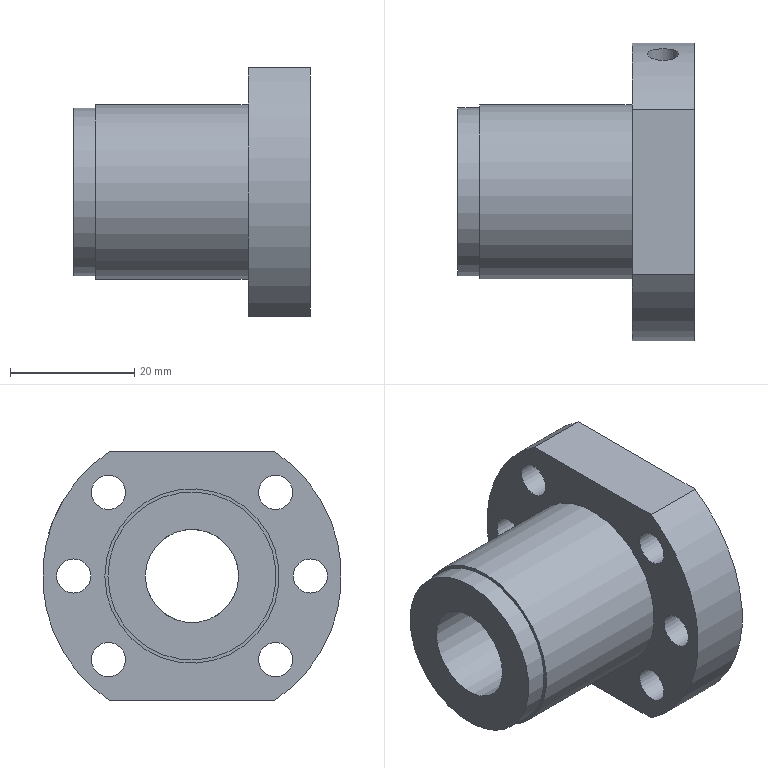Part | STEP file | 1 solid | 22 faces | box 38 x 48 x 40 mm | volume 23611 mm3 | cylinder 14 | plane 7 | cone 1 | commonest cylinder face diameters 5.5 x6 28 x2 48 x2 4 x1 4.917 x1 15 x1